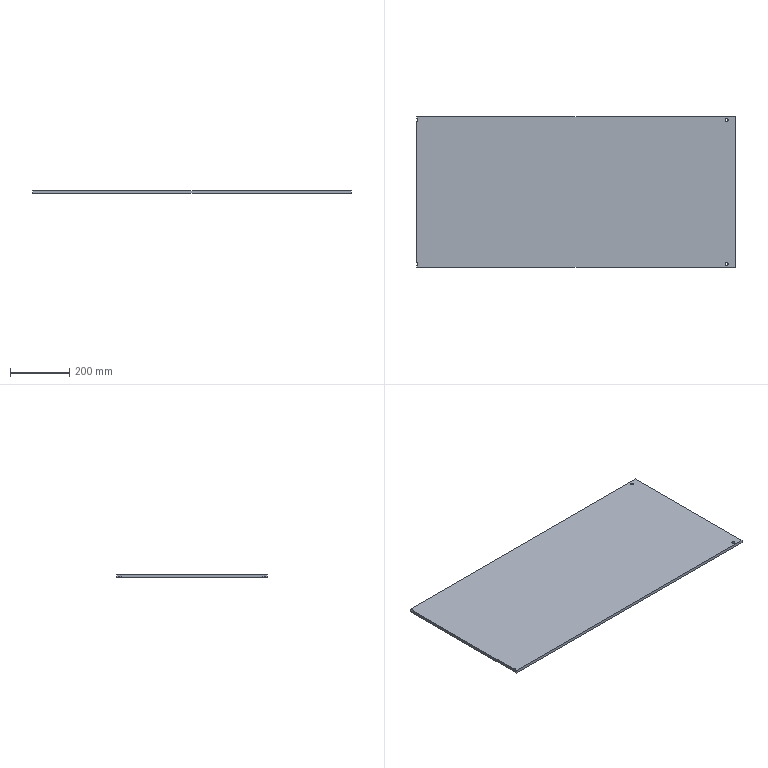Part | STEP file | 750038237 | 1 solid | 16 faces | box 1074 x 507 x 10 mm | volume 5443022 mm3 | cylinder 8 | plane 8 | commonest cylinder face diameters 10 x8
STEP:
#1=CARTESIAN_POINT('',(-537.,247.399,0.));
#2=VERTEX_POINT('',#1);
#3=CARTESIAN_POINT('',(-533.,242.5,0.));
#4=VERTEX_POINT('',#3);
#5=CARTESIAN_POINT('',(-538.,242.5,0.));
#6=DIRECTION('',(0.,0.,-1.));
#7=DIRECTION('',(1.,0.,0.));
#8=AXIS2_PLACEMENT_3D('',#5,#6,#7);
#9=CIRCLE('',#8,5.);
#10=EDGE_CURVE('',#2,#4,#9,.T.);
#11=ORIENTED_EDGE('',*,*,#10,.T.);
#12=CARTESIAN_POINT('',(-533.,242.5,10.));
#13=VERTEX_POINT('',#12);
#14=CARTESIAN_POINT('',(-533.,242.5,-1.));
#15=DIRECTION('',(0.,0.,1.));
#16=VECTOR('',#15,1000.);
#17=LINE('',#14,#16);
#18=EDGE_CURVE('',#4,#13,#17,.T.);
#19=ORIENTED_EDGE('',*,*,#18,.T.);
#20=CARTESIAN_POINT('',(-537.,247.399,10.));
#21=VERTEX_POINT('',#20);
#22=CARTESIAN_POINT('',(-538.,242.5,10.));
#23=DIRECTION('',(0.,0.,-1.));
#24=DIRECTION('',(1.,0.,0.));
#25=AXIS2_PLACEMENT_3D('',#22,#23,#24);
#26=CIRCLE('',#25,5.);
#27=EDGE_CURVE('',#21,#13,#26,.T.);
#28=ORIENTED_EDGE('',*,*,#27,.F.);
#29=CARTESIAN_POINT('',(-537.,247.399,-1.));
#30=DIRECTION('',(0.,0.,1.));
#31=VECTOR('',#30,1000.);
#32=LINE('',#29,#31);
#33=EDGE_CURVE('',#2,#21,#32,.T.);
#34=ORIENTED_EDGE('',*,*,#33,.F.);
#35=EDGE_LOOP('',(#11,#19,#28,#34));
#36=FACE_OUTER_BOUND('',#35,.T.);
#37=CARTESIAN_POINT('',(-538.,242.5,-1.));
#38=DIRECTION('',(0.,0.,1.));
#39=DIRECTION('',(1.,0.,0.));
#40=AXIS2_PLACEMENT_3D('',#37,#38,#39);
#41=CYLINDRICAL_SURFACE('',#40,5.);
#42=ADVANCED_FACE('',(#36),#41,.F.);
#43=CARTESIAN_POINT('',(-537.,-237.601,0.));
#44=VERTEX_POINT('',#43);
#45=CARTESIAN_POINT('',(-533.,-242.5,0.));
#46=VERTEX_POINT('',#45);
#47=CARTESIAN_POINT('',(-538.,-242.5,0.));
#48=DIRECTION('',(0.,0.,-1.));
#49=DIRECTION('',(1.,0.,0.));
#50=AXIS2_PLACEMENT_3D('',#47,#48,#49);
#51=CIRCLE('',#50,5.);
#52=EDGE_CURVE('',#44,#46,#51,.T.);
#53=ORIENTED_EDGE('',*,*,#52,.T.);
#54=CARTESIAN_POINT('',(-533.,-242.5,10.));
#55=VERTEX_POINT('',#54);
#56=CARTESIAN_POINT('',(-533.,-242.5,-1.));
#57=DIRECTION('',(0.,0.,1.));
#58=VECTOR('',#57,1000.);
#59=LINE('',#56,#58);
#60=EDGE_CURVE('',#46,#55,#59,.T.);
#61=ORIENTED_EDGE('',*,*,#60,.T.);
#62=CARTESIAN_POINT('',(-537.,-237.601,10.));
#63=VERTEX_POINT('',#62);
#64=CARTESIAN_POINT('',(-538.,-242.5,10.));
#65=DIRECTION('',(0.,0.,-1.));
#66=DIRECTION('',(1.,0.,0.));
#67=AXIS2_PLACEMENT_3D('',#64,#65,#66);
#68=CIRCLE('',#67,5.);
#69=EDGE_CURVE('',#63,#55,#68,.T.);
#70=ORIENTED_EDGE('',*,*,#69,.F.);
#71=CARTESIAN_POINT('',(-537.,-237.601,10.));
#72=DIRECTION('',(0.,0.,-1.));
#73=VECTOR('',#72,1000.);
#74=LINE('',#71,#73);
#75=EDGE_CURVE('',#63,#44,#74,.T.);
#76=ORIENTED_EDGE('',*,*,#75,.T.);
#77=EDGE_LOOP('',(#53,#61,#70,#76));
#78=FACE_OUTER_BOUND('',#77,.T.);
#79=CARTESIAN_POINT('',(-538.,-242.5,-1.));
#80=DIRECTION('',(0.,0.,1.));
#81=DIRECTION('',(1.,0.,0.));
#82=AXIS2_PLACEMENT_3D('',#79,#80,#81);
#83=CYLINDRICAL_SURFACE('',#82,5.);
#84=ADVANCED_FACE('',(#78),#83,.F.);
#85=CARTESIAN_POINT('',(512.,242.5,0.));
#86=VERTEX_POINT('',#85);
#87=CARTESIAN_POINT('',(502.,242.5,0.));
#88=VERTEX_POINT('',#87);
#89=CARTESIAN_POINT('',(507.,242.5,0.));
#90=DIRECTION('',(0.,0.,-1.));
#91=DIRECTION('',(1.,0.,0.));
#92=AXIS2_PLACEMENT_3D('',#89,#90,#91);
#93=CIRCLE('',#92,5.);
#94=EDGE_CURVE('',#86,#88,#93,.T.);
#95=ORIENTED_EDGE('',*,*,#94,.T.);
#96=CARTESIAN_POINT('',(502.,242.5,10.));
#97=VERTEX_POINT('',#96);
#98=CARTESIAN_POINT('',(502.,242.5,-1.));
#99=DIRECTION('',(0.,0.,1.));
#100=VECTOR('',#99,1000.);
#101=LINE('',#98,#100);
#102=EDGE_CURVE('',#88,#97,#101,.T.);
#103=ORIENTED_EDGE('',*,*,#102,.T.);
#104=CARTESIAN_POINT('',(512.,242.5,10.));
#105=VERTEX_POINT('',#104);
#106=CARTESIAN_POINT('',(507.,242.5,10.));
#107=DIRECTION('',(0.,0.,-1.));
#108=DIRECTION('',(1.,0.,0.));
#109=AXIS2_PLACEMENT_3D('',#106,#107,#108);
#110=CIRCLE('',#109,5.);
#111=EDGE_CURVE('',#105,#97,#110,.T.);
#112=ORIENTED_EDGE('',*,*,#111,.F.);
#113=CARTESIAN_POINT('',(512.,242.5,-1.));
#114=DIRECTION('',(0.,0.,1.));
#115=VECTOR('',#114,1000.);
#116=LINE('',#113,#115);
#117=EDGE_CURVE('',#86,#105,#116,.T.);
#118=ORIENTED_EDGE('',*,*,#117,.F.);
#119=EDGE_LOOP('',(#95,#103,#112,#118));
#120=FACE_OUTER_BOUND('',#119,.T.);
#121=CARTESIAN_POINT('',(507.,242.5,-1.));
#122=DIRECTION('',(0.,0.,1.));
#123=DIRECTION('',(1.,0.,0.));
#124=AXIS2_PLACEMENT_3D('',#121,#122,#123);
#125=CYLINDRICAL_SURFACE('',#124,5.);
#126=ADVANCED_FACE('',(#120),#125,.F.);
#127=CARTESIAN_POINT('',(512.,-242.5,0.));
#128=VERTEX_POINT('',#127);
#129=CARTESIAN_POINT('',(502.,-242.5,0.));
#130=VERTEX_POINT('',#129);
#131=CARTESIAN_POINT('',(507.,-242.5,0.));
#132=DIRECTION('',(0.,0.,-1.));
#133=DIRECTION('',(1.,0.,0.));
#134=AXIS2_PLACEMENT_3D('',#131,#132,#133);
#135=CIRCLE('',#134,5.);
#136=EDGE_CURVE('',#128,#130,#135,.T.);
#137=ORIENTED_EDGE('',*,*,#136,.T.);
#138=CARTESIAN_POINT('',(502.,-242.5,10.));
#139=VERTEX_POINT('',#138);
#140=CARTESIAN_POINT('',(502.,-242.5,-1.));
#141=DIRECTION('',(0.,0.,1.));
#142=VECTOR('',#141,1000.);
#143=LINE('',#140,#142);
#144=EDGE_CURVE('',#130,#139,#143,.T.);
#145=ORIENTED_EDGE('',*,*,#144,.T.);
#146=CARTESIAN_POINT('',(512.,-242.5,10.));
#147=VERTEX_POINT('',#146);
#148=CARTESIAN_POINT('',(507.,-242.5,10.));
#149=DIRECTION('',(0.,0.,-1.));
#150=DIRECTION('',(1.,0.,0.));
#151=AXIS2_PLACEMENT_3D('',#148,#149,#150);
#152=CIRCLE('',#151,5.);
#153=EDGE_CURVE('',#147,#139,#152,.T.);
#154=ORIENTED_EDGE('',*,*,#153,.F.);
#155=CARTESIAN_POINT('',(512.,-242.5,-1.));
#156=DIRECTION('',(0.,0.,1.));
#157=VECTOR('',#156,1000.);
#158=LINE('',#155,#157);
#159=EDGE_CURVE('',#128,#147,#158,.T.);
#160=ORIENTED_EDGE('',*,*,#159,.F.);
#161=EDGE_LOOP('',(#137,#145,#154,#160));
#162=FACE_OUTER_BOUND('',#161,.T.);
#163=CARTESIAN_POINT('',(507.,-242.5,-1.));
#164=DIRECTION('',(0.,0.,1.));
#165=DIRECTION('',(1.,0.,0.));
#166=AXIS2_PLACEMENT_3D('',#163,#164,#165);
#167=CYLINDRICAL_SURFACE('',#166,5.);
#168=ADVANCED_FACE('',(#162),#167,.F.);
#169=ORIENTED_EDGE('',*,*,#10,.F.);
#170=CARTESIAN_POINT('',(-537.,253.5,0.));
#171=VERTEX_POINT('',#170);
#172=CARTESIAN_POINT('',(-537.,0.,0.));
#173=DIRECTION('',(0.,-1.,0.));
#174=VECTOR('',#173,1000.);
#175=LINE('',#172,#174);
#176=EDGE_CURVE('',#171,#2,#175,.T.);
#177=ORIENTED_EDGE('',*,*,#176,.F.);
#178=CARTESIAN_POINT('',(537.,253.5,0.));
#179=VERTEX_POINT('',#178);
#180=CARTESIAN_POINT('',(0.,253.5,0.));
#181=DIRECTION('',(-1.,0.,0.));
#182=VECTOR('',#181,1000.);
#183=LINE('',#180,#182);
#184=EDGE_CURVE('',#179,#171,#183,.T.);
#185=ORIENTED_EDGE('',*,*,#184,.F.);
#186=CARTESIAN_POINT('',(537.,-253.5,0.));
#187=VERTEX_POINT('',#186);
#188=CARTESIAN_POINT('',(537.,0.,0.));
#189=DIRECTION('',(0.,1.,0.));
#190=VECTOR('',#189,1000.);
#191=LINE('',#188,#190);
#192=EDGE_CURVE('',#187,#179,#191,.T.);
#193=ORIENTED_EDGE('',*,*,#192,.F.);
#194=CARTESIAN_POINT('',(-537.,-253.5,0.));
#195=VERTEX_POINT('',#194);
#196=CARTESIAN_POINT('',(0.,-253.5,0.));
#197=DIRECTION('',(1.,0.,0.));
#198=VECTOR('',#197,1000.);
#199=LINE('',#196,#198);
#200=EDGE_CURVE('',#195,#187,#199,.T.);
#201=ORIENTED_EDGE('',*,*,#200,.F.);
#202=CARTESIAN_POINT('',(-537.,-247.399,0.));
#203=VERTEX_POINT('',#202);
#204=CARTESIAN_POINT('',(-537.,0.,0.));
#205=DIRECTION('',(0.,-1.,0.));
#206=VECTOR('',#205,1000.);
#207=LINE('',#204,#206);
#208=EDGE_CURVE('',#203,#195,#207,.T.);
#209=ORIENTED_EDGE('',*,*,#208,.F.);
#210=CARTESIAN_POINT('',(-538.,-242.5,0.));
#211=DIRECTION('',(0.,0.,-1.));
#212=DIRECTION('',(1.,0.,0.));
#213=AXIS2_PLACEMENT_3D('',#210,#211,#212);
#214=CIRCLE('',#213,5.);
#215=EDGE_CURVE('',#46,#203,#214,.T.);
#216=ORIENTED_EDGE('',*,*,#215,.F.);
#217=ORIENTED_EDGE('',*,*,#52,.F.);
#218=CARTESIAN_POINT('',(-537.,237.601,0.));
#219=VERTEX_POINT('',#218);
#220=CARTESIAN_POINT('',(-537.,0.,0.));
#221=DIRECTION('',(0.,-1.,0.));
#222=VECTOR('',#221,1000.);
#223=LINE('',#220,#222);
#224=EDGE_CURVE('',#219,#44,#223,.T.);
#225=ORIENTED_EDGE('',*,*,#224,.F.);
#226=CARTESIAN_POINT('',(-538.,242.5,0.));
#227=DIRECTION('',(0.,0.,-1.));
#228=DIRECTION('',(1.,0.,0.));
#229=AXIS2_PLACEMENT_3D('',#226,#227,#228);
#230=CIRCLE('',#229,5.);
#231=EDGE_CURVE('',#4,#219,#230,.T.);
#232=ORIENTED_EDGE('',*,*,#231,.F.);
#233=EDGE_LOOP('',(#169,#177,#185,#193,#201,#209,#216,#217,#225,#232));
#234=FACE_OUTER_BOUND('',#233,.T.);
#235=ORIENTED_EDGE('',*,*,#94,.F.);
#236=CARTESIAN_POINT('',(507.,242.5,0.));
#237=DIRECTION('',(0.,0.,-1.));
#238=DIRECTION('',(1.,0.,0.));
#239=AXIS2_PLACEMENT_3D('',#236,#237,#238);
#240=CIRCLE('',#239,5.);
#241=EDGE_CURVE('',#88,#86,#240,.T.);
#242=ORIENTED_EDGE('',*,*,#241,.F.);
#243=EDGE_LOOP('',(#235,#242));
#244=FACE_BOUND('',#243,.T.);
#245=ORIENTED_EDGE('',*,*,#136,.F.);
#246=CARTESIAN_POINT('',(507.,-242.5,0.));
#247=DIRECTION('',(0.,0.,-1.));
#248=DIRECTION('',(1.,0.,0.));
#249=AXIS2_PLACEMENT_3D('',#246,#247,#248);
#250=CIRCLE('',#249,5.);
#251=EDGE_CURVE('',#130,#128,#250,.T.);
#252=ORIENTED_EDGE('',*,*,#251,.F.);
#253=EDGE_LOOP('',(#245,#252));
#254=FACE_BOUND('',#253,.T.);
#255=CARTESIAN_POINT('',(0.,0.,0.));
#256=DIRECTION('',(0.,0.,1.));
#257=DIRECTION('',(1.,0.,0.));
#258=AXIS2_PLACEMENT_3D('',#255,#256,#257);
#259=PLANE('',#258);
#260=ADVANCED_FACE('',(#234,#244,#254),#259,.F.);
#261=CARTESIAN_POINT('',(-537.,237.601,10.));
#262=VERTEX_POINT('',#261);
#263=CARTESIAN_POINT('',(-537.,237.601,10.));
#264=DIRECTION('',(0.,0.,1.));
#265=VECTOR('',#264,1000.);
#266=LINE('',#263,#265);
#267=EDGE_CURVE('',#219,#262,#266,.T.);
#268=ORIENTED_EDGE('',*,*,#267,.F.);
#269=ORIENTED_EDGE('',*,*,#224,.T.);
#270=ORIENTED_EDGE('',*,*,#75,.F.);
#271=CARTESIAN_POINT('',(-537.,253.5,10.));
#272=DIRECTION('',(0.,-1.,0.));
#273=VECTOR('',#272,1000.);
#274=LINE('',#271,#273);
#275=EDGE_CURVE('',#262,#63,#274,.T.);
#276=ORIENTED_EDGE('',*,*,#275,.F.);
#277=EDGE_LOOP('',(#268,#269,#270,#276));
#278=FACE_OUTER_BOUND('',#277,.T.);
#279=CARTESIAN_POINT('',(-537.,253.5,10.));
#280=DIRECTION('',(1.,0.,0.));
#281=DIRECTION('',(0.,0.,-1.));
#282=AXIS2_PLACEMENT_3D('',#279,#280,#281);
#283=PLANE('',#282);
#284=ADVANCED_FACE('',(#278),#283,.F.);
#285=ORIENTED_EDGE('',*,*,#18,.F.);
#286=ORIENTED_EDGE('',*,*,#231,.T.);
#287=ORIENTED_EDGE('',*,*,#267,.T.);
#288=CARTESIAN_POINT('',(-538.,242.5,10.));
#289=DIRECTION('',(0.,0.,-1.));
#290=DIRECTION('',(1.,0.,0.));
#291=AXIS2_PLACEMENT_3D('',#288,#289,#290);
#292=CIRCLE('',#291,5.);
#293=EDGE_CURVE('',#13,#262,#292,.T.);
#294=ORIENTED_EDGE('',*,*,#293,.F.);
#295=EDGE_LOOP('',(#285,#286,#287,#294));
#296=FACE_OUTER_BOUND('',#295,.T.);
#297=CARTESIAN_POINT('',(-538.,242.5,-1.));
#298=DIRECTION('',(0.,0.,1.));
#299=DIRECTION('',(1.,0.,0.));
#300=AXIS2_PLACEMENT_3D('',#297,#298,#299);
#301=CYLINDRICAL_SURFACE('',#300,5.);
#302=ADVANCED_FACE('',(#296),#301,.F.);
#303=ORIENTED_EDGE('',*,*,#33,.T.);
#304=CARTESIAN_POINT('',(-537.,253.5,10.));
#305=VERTEX_POINT('',#304);
#306=CARTESIAN_POINT('',(-537.,253.5,10.));
#307=DIRECTION('',(0.,-1.,0.));
#308=VECTOR('',#307,1000.);
#309=LINE('',#306,#308);
#310=EDGE_CURVE('',#305,#21,#309,.T.);
#311=ORIENTED_EDGE('',*,*,#310,.F.);
#312=CARTESIAN_POINT('',(-537.,253.5,10.));
#313=DIRECTION('',(0.,0.,1.));
#314=VECTOR('',#313,1000.);
#315=LINE('',#312,#314);
#316=EDGE_CURVE('',#171,#305,#315,.T.);
#317=ORIENTED_EDGE('',*,*,#316,.F.);
#318=ORIENTED_EDGE('',*,*,#176,.T.);
#319=EDGE_LOOP('',(#303,#311,#317,#318));
#320=FACE_OUTER_BOUND('',#319,.T.);
#321=CARTESIAN_POINT('',(-537.,253.5,10.));
#322=DIRECTION('',(1.,0.,0.));
#323=DIRECTION('',(0.,0.,-1.));
#324=AXIS2_PLACEMENT_3D('',#321,#322,#323);
#325=PLANE('',#324);
#326=ADVANCED_FACE('',(#320),#325,.F.);
#327=ORIENTED_EDGE('',*,*,#316,.T.);
#328=CARTESIAN_POINT('',(537.,253.5,10.));
#329=VERTEX_POINT('',#328);
#330=CARTESIAN_POINT('',(537.,253.5,10.));
#331=DIRECTION('',(-1.,0.,0.));
#332=VECTOR('',#331,1000.);
#333=LINE('',#330,#332);
#334=EDGE_CURVE('',#329,#305,#333,.T.);
#335=ORIENTED_EDGE('',*,*,#334,.F.);
#336=CARTESIAN_POINT('',(537.,253.5,10.));
#337=DIRECTION('',(0.,0.,1.));
#338=VECTOR('',#337,1000.);
#339=LINE('',#336,#338);
#340=EDGE_CURVE('',#179,#329,#339,.T.);
#341=ORIENTED_EDGE('',*,*,#340,.F.);
#342=ORIENTED_EDGE('',*,*,#184,.T.);
#343=EDGE_LOOP('',(#327,#335,#341,#342));
#344=FACE_OUTER_BOUND('',#343,.T.);
#345=CARTESIAN_POINT('',(537.,253.5,10.));
#346=DIRECTION('',(0.,-1.,0.));
#347=DIRECTION('',(0.,0.,-1.));
#348=AXIS2_PLACEMENT_3D('',#345,#346,#347);
#349=PLANE('',#348);
#350=ADVANCED_FACE('',(#344),#349,.F.);
#351=ORIENTED_EDGE('',*,*,#340,.T.);
#352=CARTESIAN_POINT('',(537.,-253.5,10.));
#353=VERTEX_POINT('',#352);
#354=CARTESIAN_POINT('',(537.,-253.5,10.));
#355=DIRECTION('',(0.,1.,0.));
#356=VECTOR('',#355,1000.);
#357=LINE('',#354,#356);
#358=EDGE_CURVE('',#353,#329,#357,.T.);
#359=ORIENTED_EDGE('',*,*,#358,.F.);
#360=CARTESIAN_POINT('',(537.,-253.5,10.));
#361=DIRECTION('',(0.,0.,1.));
#362=VECTOR('',#361,1000.);
#363=LINE('',#360,#362);
#364=EDGE_CURVE('',#187,#353,#363,.T.);
#365=ORIENTED_EDGE('',*,*,#364,.F.);
#366=ORIENTED_EDGE('',*,*,#192,.T.);
#367=EDGE_LOOP('',(#351,#359,#365,#366));
#368=FACE_OUTER_BOUND('',#367,.T.);
#369=CARTESIAN_POINT('',(537.,-253.5,10.));
#370=DIRECTION('',(-1.,0.,0.));
#371=DIRECTION('',(0.,0.,1.));
#372=AXIS2_PLACEMENT_3D('',#369,#370,#371);
#373=PLANE('',#372);
#374=ADVANCED_FACE('',(#368),#373,.F.);
#375=ORIENTED_EDGE('',*,*,#364,.T.);
#376=CARTESIAN_POINT('',(-537.,-253.5,10.));
#377=VERTEX_POINT('',#376);
#378=CARTESIAN_POINT('',(-537.,-253.5,10.));
#379=DIRECTION('',(1.,0.,0.));
#380=VECTOR('',#379,1000.);
#381=LINE('',#378,#380);
#382=EDGE_CURVE('',#377,#353,#381,.T.);
#383=ORIENTED_EDGE('',*,*,#382,.F.);
#384=CARTESIAN_POINT('',(-537.,-253.5,10.));
#385=DIRECTION('',(0.,0.,1.));
#386=VECTOR('',#385,1000.);
#387=LINE('',#384,#386);
#388=EDGE_CURVE('',#195,#377,#387,.T.);
#389=ORIENTED_EDGE('',*,*,#388,.F.);
#390=ORIENTED_EDGE('',*,*,#200,.T.);
#391=EDGE_LOOP('',(#375,#383,#389,#390));
#392=FACE_OUTER_BOUND('',#391,.T.);
#393=CARTESIAN_POINT('',(-537.,-253.5,10.));
#394=DIRECTION('',(0.,1.,0.));
#395=DIRECTION('',(0.,0.,1.));
#396=AXIS2_PLACEMENT_3D('',#393,#394,#395);
#397=PLANE('',#396);
#398=ADVANCED_FACE('',(#392),#397,.F.);
#399=CARTESIAN_POINT('',(-537.,-247.399,10.));
#400=VERTEX_POINT('',#399);
#401=CARTESIAN_POINT('',(-537.,-247.399,10.));
#402=DIRECTION('',(0.,0.,1.));
#403=VECTOR('',#402,1000.);
#404=LINE('',#401,#403);
#405=EDGE_CURVE('',#203,#400,#404,.T.);
#406=ORIENTED_EDGE('',*,*,#405,.F.);
#407=ORIENTED_EDGE('',*,*,#208,.T.);
#408=ORIENTED_EDGE('',*,*,#388,.T.);
#409=CARTESIAN_POINT('',(-537.,253.5,10.));
#410=DIRECTION('',(0.,-1.,0.));
#411=VECTOR('',#410,1000.);
#412=LINE('',#409,#411);
#413=EDGE_CURVE('',#400,#377,#412,.T.);
#414=ORIENTED_EDGE('',*,*,#413,.F.);
#415=EDGE_LOOP('',(#406,#407,#408,#414));
#416=FACE_OUTER_BOUND('',#415,.T.);
#417=CARTESIAN_POINT('',(-537.,253.5,10.));
#418=DIRECTION('',(1.,0.,0.));
#419=DIRECTION('',(0.,0.,-1.));
#420=AXIS2_PLACEMENT_3D('',#417,#418,#419);
#421=PLANE('',#420);
#422=ADVANCED_FACE('',(#416),#421,.F.);
#423=ORIENTED_EDGE('',*,*,#60,.F.);
#424=ORIENTED_EDGE('',*,*,#215,.T.);
#425=ORIENTED_EDGE('',*,*,#405,.T.);
#426=CARTESIAN_POINT('',(-538.,-242.5,10.));
#427=DIRECTION('',(0.,0.,-1.));
#428=DIRECTION('',(1.,0.,0.));
#429=AXIS2_PLACEMENT_3D('',#426,#427,#428);
#430=CIRCLE('',#429,5.);
#431=EDGE_CURVE('',#55,#400,#430,.T.);
#432=ORIENTED_EDGE('',*,*,#431,.F.);
#433=EDGE_LOOP('',(#423,#424,#425,#432));
#434=FACE_OUTER_BOUND('',#433,.T.);
#435=CARTESIAN_POINT('',(-538.,-242.5,-1.));
#436=DIRECTION('',(0.,0.,1.));
#437=DIRECTION('',(1.,0.,0.));
#438=AXIS2_PLACEMENT_3D('',#435,#436,#437);
#439=CYLINDRICAL_SURFACE('',#438,5.);
#440=ADVANCED_FACE('',(#434),#439,.F.);
#441=ORIENTED_EDGE('',*,*,#102,.F.);
#442=ORIENTED_EDGE('',*,*,#241,.T.);
#443=ORIENTED_EDGE('',*,*,#117,.T.);
#444=CARTESIAN_POINT('',(507.,242.5,10.));
#445=DIRECTION('',(0.,0.,-1.));
#446=DIRECTION('',(1.,0.,0.));
#447=AXIS2_PLACEMENT_3D('',#444,#445,#446);
#448=CIRCLE('',#447,5.);
#449=EDGE_CURVE('',#97,#105,#448,.T.);
#450=ORIENTED_EDGE('',*,*,#449,.F.);
#451=EDGE_LOOP('',(#441,#442,#443,#450));
#452=FACE_OUTER_BOUND('',#451,.T.);
#453=CARTESIAN_POINT('',(507.,242.5,-1.));
#454=DIRECTION('',(0.,0.,1.));
#455=DIRECTION('',(1.,0.,0.));
#456=AXIS2_PLACEMENT_3D('',#453,#454,#455);
#457=CYLINDRICAL_SURFACE('',#456,5.);
#458=ADVANCED_FACE('',(#452),#457,.F.);
#459=ORIENTED_EDGE('',*,*,#144,.F.);
#460=ORIENTED_EDGE('',*,*,#251,.T.);
#461=ORIENTED_EDGE('',*,*,#159,.T.);
#462=CARTESIAN_POINT('',(507.,-242.5,10.));
#463=DIRECTION('',(0.,0.,-1.));
#464=DIRECTION('',(1.,0.,0.));
#465=AXIS2_PLACEMENT_3D('',#462,#463,#464);
#466=CIRCLE('',#465,5.);
#467=EDGE_CURVE('',#139,#147,#466,.T.);
#468=ORIENTED_EDGE('',*,*,#467,.F.);
#469=EDGE_LOOP('',(#459,#460,#461,#468));
#470=FACE_OUTER_BOUND('',#469,.T.);
#471=CARTESIAN_POINT('',(507.,-242.5,-1.));
#472=DIRECTION('',(0.,0.,1.));
#473=DIRECTION('',(1.,0.,0.));
#474=AXIS2_PLACEMENT_3D('',#471,#472,#473);
#475=CYLINDRICAL_SURFACE('',#474,5.);
#476=ADVANCED_FACE('',(#470),#475,.F.);
#477=ORIENTED_EDGE('',*,*,#111,.T.);
#478=ORIENTED_EDGE('',*,*,#449,.T.);
#479=EDGE_LOOP('',(#477,#478));
#480=FACE_BOUND('',#479,.T.);
#481=ORIENTED_EDGE('',*,*,#334,.T.);
#482=ORIENTED_EDGE('',*,*,#310,.T.);
#483=ORIENTED_EDGE('',*,*,#27,.T.);
#484=ORIENTED_EDGE('',*,*,#293,.T.);
#485=ORIENTED_EDGE('',*,*,#275,.T.);
#486=ORIENTED_EDGE('',*,*,#69,.T.);
#487=ORIENTED_EDGE('',*,*,#431,.T.);
#488=ORIENTED_EDGE('',*,*,#413,.T.);
#489=ORIENTED_EDGE('',*,*,#382,.T.);
#490=ORIENTED_EDGE('',*,*,#358,.T.);
#491=EDGE_LOOP('',(#481,#482,#483,#484,#485,#486,#487,#488,#489,#490));
#492=FACE_OUTER_BOUND('',#491,.T.);
#493=ORIENTED_EDGE('',*,*,#153,.T.);
#494=ORIENTED_EDGE('',*,*,#467,.T.);
#495=EDGE_LOOP('',(#493,#494));
#496=FACE_BOUND('',#495,.T.);
#497=CARTESIAN_POINT('',(0.,0.,10.));
#498=DIRECTION('',(0.,0.,1.));
#499=DIRECTION('',(1.,0.,0.));
#500=AXIS2_PLACEMENT_3D('',#497,#498,#499);
#501=PLANE('',#500);
#502=ADVANCED_FACE('',(#480,#492,#496),#501,.T.);
#503=CLOSED_SHELL('',(#42,#84,#126,#168,#260,#284,#302,#326,#350,#374,#398,#422,#440,#458,#476,#502));
#504=MANIFOLD_SOLID_BREP('',#503);
#505=CARTESIAN_POINT('',(0.,0.,0.));
#506=DIRECTION('',(0.,0.,1.));
#507=DIRECTION('',(1.,0.,0.));
#508=AXIS2_PLACEMENT_3D('',#505,#506,#507);
#509=(LENGTH_UNIT()NAMED_UNIT(*)SI_UNIT(.MILLI.,.METRE.));
#510=UNCERTAINTY_MEASURE_WITH_UNIT(LENGTH_MEASURE(0.00001),#509,'','');
#511=(NAMED_UNIT(*)PLANE_ANGLE_UNIT()SI_UNIT($,.RADIAN.));
#512=(NAMED_UNIT(*)SI_UNIT($,.STERADIAN.)SOLID_ANGLE_UNIT());
#513=(GEOMETRIC_REPRESENTATION_CONTEXT(3)GLOBAL_UNCERTAINTY_ASSIGNED_CONTEXT((#510))GLOBAL_UNIT_ASSIGNED_CONTEXT((#509,#511,#512))REPRESENTATION_CONTEXT('',''));
#514=ADVANCED_BREP_SHAPE_REPRESENTATION('',(#504,#508),#513);